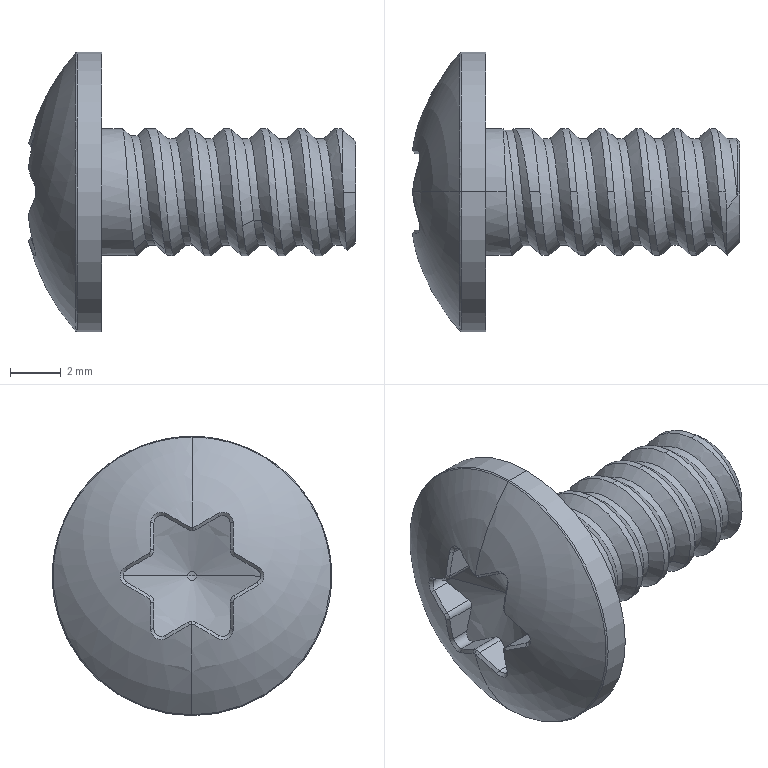Part | SolidWorks | features BaseBody 1 | 1 solid | 87 faces | box 12.881 x 11 x 11.001 mm | volume 347.163 mm3 | cylinder 27 | spline 23 | cone 17 | plane 14 | sphere 4 | torus 2 | commonest cylinder face diameters 5 x13 0.6 x12 11 x2